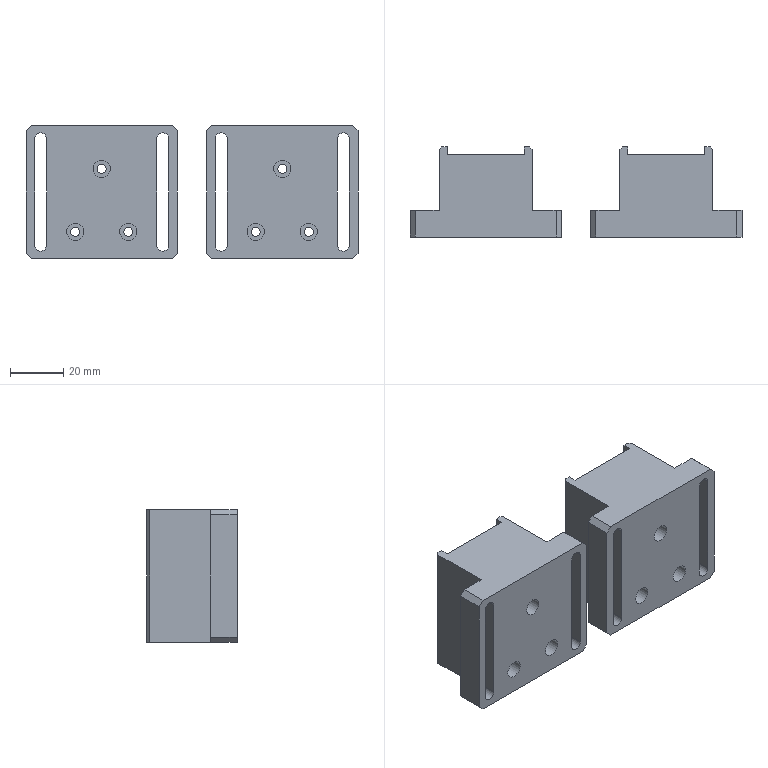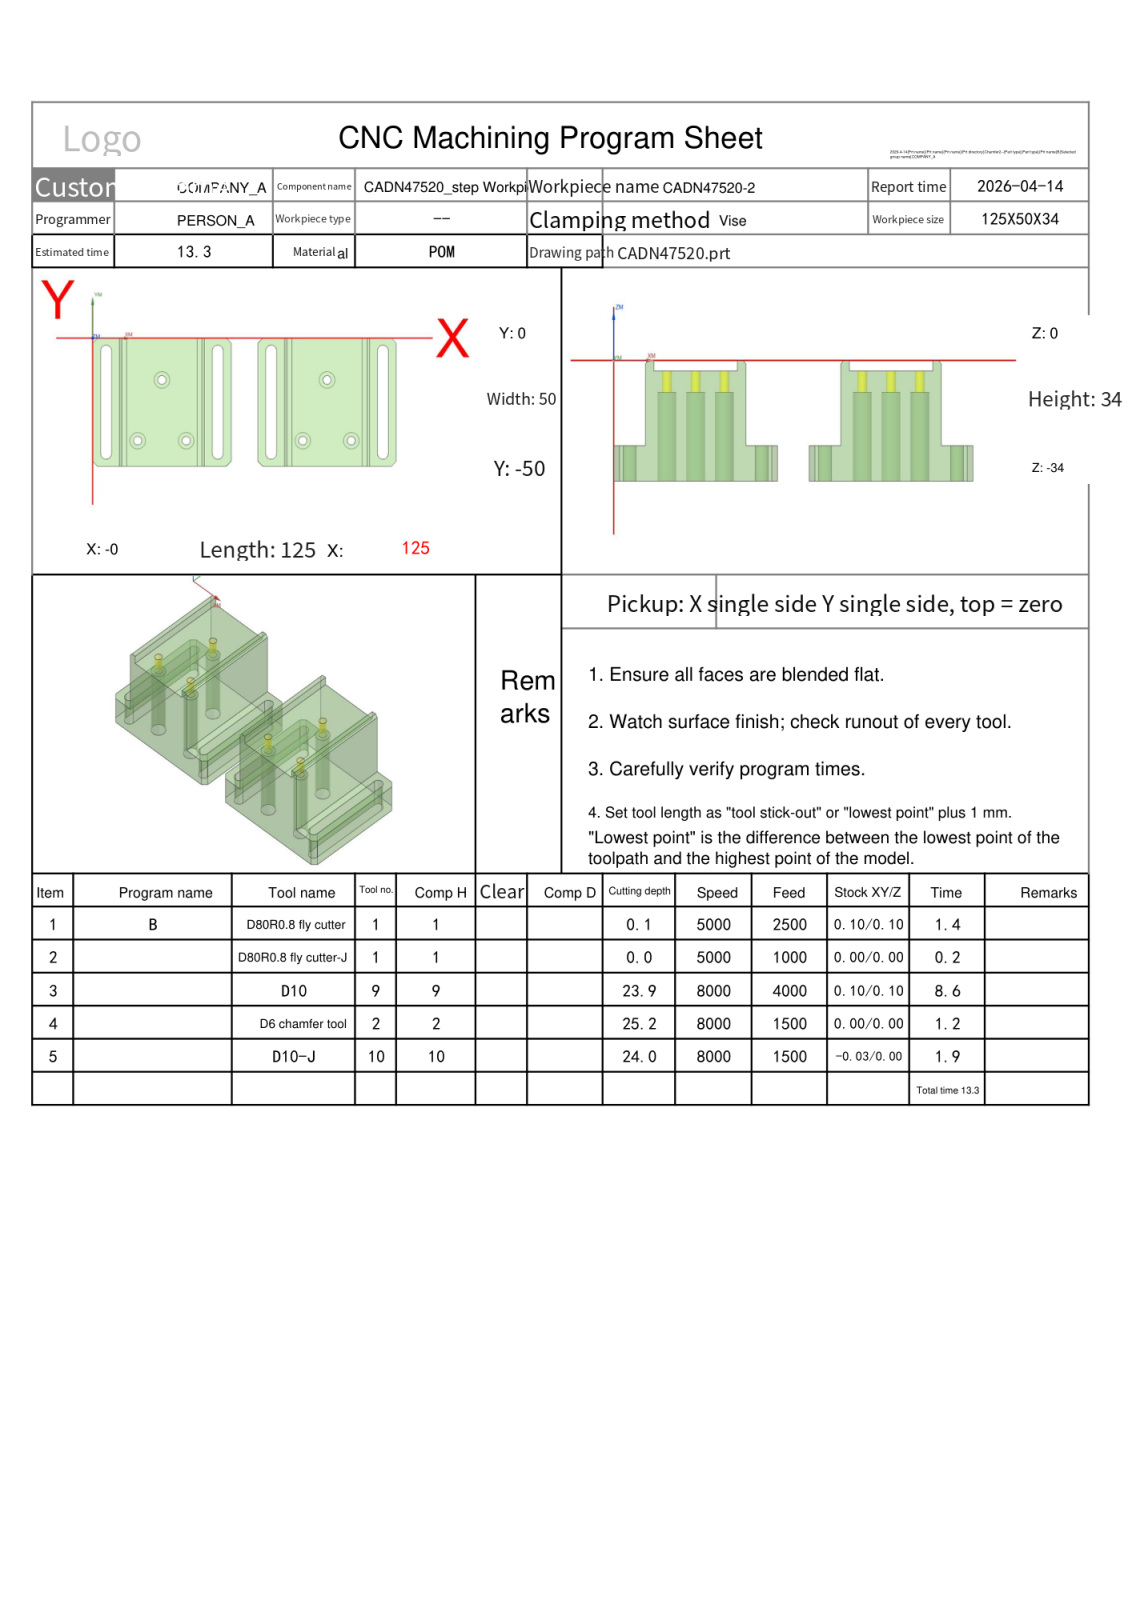NC program | NX | posted by the shop | part box 125 x 34 x 50 mm
Lines 133 to 1886 of 4293:
N3 T09 M06
(D10  D=10. R=0. H=09 ce=0.10 di=0.10)
G00 G90 G54 X28.5 Y-58. M03 S8000
G43 H09 Z15.8
M08
Z.92
G01 Z-.58 F4000.
Y-54.9
X19.1
Y4.9
X37.9
Y-54.9
X31.644
G02 X30.734 Y-54.313 I0.0 J1.
G01 X27.806 Y-47.858
G03 X27.248 Y-47.336 I-.91 J-.414
G02 X26.6 Y-46.402 I.352 J.936
G01 Y-3.598
G02 X27.598 Y-2.6 I1. J-.002
G01 X29.402
G02 X30.4 Y-3.598 I-.002 J-1.
G01 Y-46.402
G02 X29.402 Y-47.4 I-1. J.002
G01 X28.5
X28.
Y-50.4
Y-58.
Z.92
G00 X28.5
Z.34
G01 Z-1.16
Y-54.9
X19.1
Y4.9
X37.9
Y-54.9
X31.644
G02 X30.734 Y-54.313 I0.0 J1.
G01 X27.806 Y-47.858
G03 X27.248 Y-47.336 I-.91 J-.414
G02 X26.6 Y-46.402 I.352 J.936
G01 Y-3.598
G02 X27.598 Y-2.6 I1. J-.002
G01 X29.402
G02 X30.4 Y-3.598 I-.002 J-1.
G01 Y-46.402
G02 X29.402 Y-47.4 I-1. J.002
G01 X28.5
X28.
Y-50.4
Y-58.
Z.34
G00 X28.5
Z-.24
G01 Z-1.74
Y-54.9
X19.1
Y4.9
X37.9
Y-54.9
X31.644
G02 X30.734 Y-54.313 I0.0 J1.
G01 X27.806 Y-47.858
G03 X27.248 Y-47.336 I-.91 J-.414
G02 X26.6 Y-46.402 I.352 J.936
G01 Y-3.598
G02 X27.598 Y-2.6 I1. J-.002
G01 X29.402
G02 X30.4 Y-3.598 I-.002 J-1.
G01 Y-46.402
G02 X29.402 Y-47.4 I-1. J.002
G01 X28.5
X28.
Y-50.4
Y-58.
Z-.24
G00 X28.5
Z-.82
G01 Z-2.32
Y-54.9
X19.1
Y4.9
X37.9
Y-54.9
X31.644
G02 X30.734 Y-54.313 I0.0 J1.
G01 X27.806 Y-47.858
G03 X27.248 Y-47.336 I-.91 J-.414
G02 X26.6 Y-46.402 I.352 J.936
G01 Y-3.598
G02 X27.598 Y-2.6 I1. J-.002
G01 X29.402
G02 X30.4 Y-3.598 I-.002 J-1.
G01 Y-46.402
G02 X29.402 Y-47.4 I-1. J.002
G01 X28.5
X28.
Y-50.4
Y-58.
Z-.82
G00 X28.5
Z-1.4
G01 Z-2.9
Y-54.9
X19.1
Y4.9
X37.9
Y-54.9
X31.644
G02 X30.734 Y-54.313 I0.0 J1.
G01 X27.806 Y-47.858
G03 X27.248 Y-47.336 I-.91 J-.414
G02 X26.6 Y-46.402 I.352 J.936
G01 Y-3.598
G02 X27.598 Y-2.6 I1. J-.002
G01 X29.402
G02 X30.4 Y-3.598 I-.002 J-1.
G01 Y-46.402
G02 X29.402 Y-47.4 I-1. J.002
G01 X28.5
X28.
Y-50.4
Y-58.
Z-1.4
G00 Z3.
X96.5
Z.92
G01 Z-.58
Y-54.9
X87.1
Y4.9
X105.9
Y-54.9
X99.644
G02 X98.734 Y-54.313 I0.0 J1.
G01 X95.806 Y-47.858
G03 X95.248 Y-47.336 I-.91 J-.414
G02 X94.6 Y-46.402 I.352 J.936
G01 Y-3.598
G02 X95.598 Y-2.6 I1. J-.002
G01 X97.402
G02 X98.4 Y-3.598 I-.002 J-1.
G01 Y-46.402
G02 X97.402 Y-47.4 I-1. J.002
G01 X96.5
X96.
Y-50.4
Y-58.
Z.92
G00 X96.5
Z.34
G01 Z-1.16
Y-54.9
X87.1
Y4.9
X105.9
Y-54.9
X99.644
G02 X98.734 Y-54.313 I0.0 J1.
G01 X95.806 Y-47.858
G03 X95.248 Y-47.336 I-.91 J-.414
G02 X94.6 Y-46.402 I.352 J.936
G01 Y-3.598
G02 X95.598 Y-2.6 I1. J-.002
G01 X97.402
G02 X98.4 Y-3.598 I-.002 J-1.
G01 Y-46.402
G02 X97.402 Y-47.4 I-1. J.002
G01 X96.5
X96.
Y-50.4
Y-58.
Z.34
G00 X96.5
Z-.24
G01 Z-1.74
Y-54.9
X87.1
Y4.9
X105.9
Y-54.9
X99.644
G02 X98.734 Y-54.313 I0.0 J1.
G01 X95.806 Y-47.858
G03 X95.248 Y-47.336 I-.91 J-.414
G02 X94.6 Y-46.402 I.352 J.936
G01 Y-3.598
G02 X95.598 Y-2.6 I1. J-.002
G01 X97.402
G02 X98.4 Y-3.598 I-.002 J-1.
G01 Y-46.402
G02 X97.402 Y-47.4 I-1. J.002
G01 X96.5
X96.
Y-50.4
Y-58.
Z-.24
G00 X96.5
Z-.82
G01 Z-2.32
Y-54.9
X87.1
Y4.9
X105.9
Y-54.9
X99.644
G02 X98.734 Y-54.313 I0.0 J1.
G01 X95.806 Y-47.858
G03 X95.248 Y-47.336 I-.91 J-.414
G02 X94.6 Y-46.402 I.352 J.936
G01 Y-3.598
G02 X95.598 Y-2.6 I1. J-.002
G01 X97.402
G02 X98.4 Y-3.598 I-.002 J-1.
G01 Y-46.402
G02 X97.402 Y-47.4 I-1. J.002
G01 X96.5
X96.
Y-50.4
Y-58.
Z-.82
G00 X96.5
Z-1.4
G01 Z-2.9
Y-54.9
X87.1
Y4.9
X105.9
Y-54.9
X99.644
G02 X98.734 Y-54.313 I0.0 J1.
G01 X95.806 Y-47.858
G03 X95.248 Y-47.336 I-.91 J-.414
G02 X94.6 Y-46.402 I.352 J.936
G01 Y-3.598
G02 X95.598 Y-2.6 I1. J-.002
G01 X97.402
G02 X98.4 Y-3.598 I-.002 J-1.
G01 Y-46.402
G02 X97.402 Y-47.4 I-1. J.002
G01 X96.5
X96.
Y-50.4
Y-58.
Z-1.4
G00 Z15.8
G00 G90 X-8. Y-25. M03 S8000
Z15.8
Z.903
G01 Z-.598 F4000.
X-4.9
Y.03
X-.03 Y4.9
X5.9
Y-54.9
X-.03
X-4.9 Y-50.03
Y-27.664
G02 X-4.607 Y-26.957 I1. J0.0
G01 X-.693 Y-23.043
G03 X-.4 Y-22.336 I-.707 J.707
G01 Y-2.205
G02 X.5 Y-1.307 I.9 J-.002
X1.4 Y-2.205 I0.0 J-.9
G01 Y-47.795
G02 X.5 Y-48.693 I-.9 J.002
X-.4 Y-47.795 I0.0 J.9
G01 Y-25.
Y-24.5
X-8.
Z.903
G00 Y-25.
Z.305
G01 Z-1.195
X-4.9
Y.03
X-.03 Y4.9
X5.9
Y-54.9
X-.03
X-4.9 Y-50.03
Y-27.664
G02 X-4.607 Y-26.957 I1. J0.0
G01 X-.693 Y-23.043
G03 X-.4 Y-22.336 I-.707 J.707
G01 Y-2.205
G02 X.5 Y-1.307 I.9 J-.002
X1.4 Y-2.205 I0.0 J-.9
G01 Y-47.795
G02 X.5 Y-48.693 I-.9 J.002
X-.4 Y-47.795 I0.0 J.9
G01 Y-25.
Y-24.5
X-8.
Z.305
G00 Y-25.
Z-.293
G01 Z-1.793
X-4.9
Y.03
X-.03 Y4.9
X5.9
Y-54.9
X-.03
X-4.9 Y-50.03
Y-27.664
G02 X-4.607 Y-26.957 I1. J0.0
G01 X-.693 Y-23.043
G03 X-.4 Y-22.336 I-.707 J.707
G01 Y-2.205
G02 X.5 Y-1.307 I.9 J-.002
X1.4 Y-2.205 I0.0 J-.9
G01 Y-47.795
G02 X.5 Y-48.693 I-.9 J.002
X-.4 Y-47.795 I0.0 J.9
G01 Y-25.
Y-24.5
X-8.
Z-.293
G00 Y-25.
Z-.89
G01 Z-2.39
X-4.9
Y.03
X-.03 Y4.9
X5.9
Y-54.9
X-.03
X-4.9 Y-50.03
Y-27.664
G02 X-4.607 Y-26.957 I1. J0.0
G01 X-.693 Y-23.043
G03 X-.4 Y-22.336 I-.707 J.707
G01 Y-2.205
G02 X.5 Y-1.307 I.9 J-.002
X1.4 Y-2.205 I0.0 J-.9
G01 Y-47.795
G02 X.5 Y-48.693 I-.9 J.002
X-.4 Y-47.795 I0.0 J.9
G01 Y-25.
Y-24.5
X-8.
Z-.89
G00 Y-25.
Z-1.488
G01 Z-2.988
X-4.9
Y.03
X-.03 Y4.9
X5.9
Y-54.9
X-.03
X-4.9 Y-50.03
Y-27.664
G02 X-4.607 Y-26.957 I1. J0.0
G01 X-.693 Y-23.043
G03 X-.4 Y-22.336 I-.707 J.707
G01 Y-2.205
G02 X.5 Y-1.307 I.9 J-.002
X1.4 Y-2.205 I0.0 J-.9
G01 Y-47.795
G02 X.5 Y-48.693 I-.9 J.002
X-.4 Y-47.795 I0.0 J.9
G01 Y-25.
Y-24.5
X-8.
Z-1.488
G00 Y-25.
Z-2.085
G01 Z-3.585
X-4.9
Y.03
X-.03 Y4.9
X5.9
Y-54.9
X-.03
X-4.9 Y-50.03
Y-27.664
G02 X-4.607 Y-26.957 I1. J0.0
G01 X-.693 Y-23.043
G03 X-.4 Y-22.336 I-.707 J.707
G01 Y-2.205
G02 X.5 Y-1.307 I.9 J-.002
X1.4 Y-2.205 I0.0 J-.9
G01 Y-47.795
G02 X.5 Y-48.693 I-.9 J.002
X-.4 Y-47.795 I0.0 J.9
G01 Y-25.
Y-24.5
X-8.
Z-2.085
G00 Y-25.
Z-2.683
G01 Z-4.183
X-4.9
Y.03
X-.03 Y4.9
X5.9
Y-54.9
X-.03
X-4.9 Y-50.03
Y-27.664
G02 X-4.607 Y-26.957 I1. J0.0
G01 X-.693 Y-23.043
G03 X-.4 Y-22.336 I-.707 J.707
G01 Y-2.205
G02 X.5 Y-1.307 I.9 J-.002
X1.4 Y-2.205 I0.0 J-.9
G01 Y-47.795
G02 X.5 Y-48.693 I-.9 J.002
X-.4 Y-47.795 I0.0 J.9
G01 Y-25.
Y-24.5
X-8.
Z-2.683
G00 Y-25.
Z-3.28
G01 Z-4.78
X-4.9
Y.03
X-.03 Y4.9
X5.9
Y-54.9
X-.03
X-4.9 Y-50.03
Y-27.664
G02 X-4.607 Y-26.957 I1. J0.0
G01 X-.693 Y-23.043
G03 X-.4 Y-22.336 I-.707 J.707
G01 Y-2.205
G02 X.5 Y-1.307 I.9 J-.002
X1.4 Y-2.205 I0.0 J-.9
G01 Y-47.795
G02 X.5 Y-48.693 I-.9 J.002
X-.4 Y-47.795 I0.0 J.9
G01 Y-25.
Y-24.5
X-8.
Z-3.28
G00 Y-25.
Z-3.878
G01 Z-5.378
X-4.9
Y.03
X-.03 Y4.9
X5.9
Y-54.9
X-.03
X-4.9 Y-50.03
Y-27.664
G02 X-4.607 Y-26.957 I1. J0.0
G01 X-.693 Y-23.043
G03 X-.4 Y-22.336 I-.707 J.707
G01 Y-2.205
G02 X.5 Y-1.307 I.9 J-.002
X1.4 Y-2.205 I0.0 J-.9
G01 Y-47.795
G02 X.5 Y-48.693 I-.9 J.002
X-.4 Y-47.795 I0.0 J.9
G01 Y-25.
Y-24.5
X-8.
Z-3.878
G00 Y-25.
Z-4.475
G01 Z-5.975
X-4.9
Y.03
X-.03 Y4.9
X5.9
Y-54.9
X-.03
X-4.9 Y-50.03
Y-27.664
G02 X-4.607 Y-26.957 I1. J0.0
G01 X-.693 Y-23.043
G03 X-.4 Y-22.336 I-.707 J.707
G01 Y-2.205
G02 X.5 Y-1.307 I.9 J-.002
X1.4 Y-2.205 I0.0 J-.9
G01 Y-47.795
G02 X.5 Y-48.693 I-.9 J.002
X-.4 Y-47.795 I0.0 J.9
G01 Y-25.
Y-24.5
X-8.
Z-4.475
G00 Y-25.
Z-5.073
G01 Z-6.573
X-4.9
Y.03
X-.03 Y4.9
X5.9
Y-54.9
X-.03
X-4.9 Y-50.03
Y-27.664
G02 X-4.607 Y-26.957 I1. J0.0
G01 X-.693 Y-23.043
G03 X-.4 Y-22.336 I-.707 J.707
G01 Y-2.205
G02 X.5 Y-1.307 I.9 J-.002
X1.4 Y-2.205 I0.0 J-.9
G01 Y-47.795
G02 X.5 Y-48.693 I-.9 J.002
X-.4 Y-47.795 I0.0 J.9
G01 Y-25.
Y-24.5
X-8.
Z-5.073
G00 Y-25.
Z-5.67
G01 Z-7.17
X-4.9
Y.03
X-.03 Y4.9
X5.9
Y-54.9
X-.03
X-4.9 Y-50.03
Y-27.664
G02 X-4.607 Y-26.957 I1. J0.0
G01 X-.693 Y-23.043
G03 X-.4 Y-22.336 I-.707 J.707
G01 Y-2.205
G02 X.5 Y-1.307 I.9 J-.002
X1.4 Y-2.205 I0.0 J-.9
G01 Y-47.795
G02 X.5 Y-48.693 I-.9 J.002
X-.4 Y-47.795 I0.0 J.9
G01 Y-25.
Y-24.5
X-8.
Z-5.67
G00 Y-25.
Z-6.268
G01 Z-7.768
X-4.9
Y.03
X-.03 Y4.9
X5.9
Y-54.9
X-.03
X-4.9 Y-50.03
Y-27.664
G02 X-4.607 Y-26.957 I1. J0.0
G01 X-.693 Y-23.043
G03 X-.4 Y-22.336 I-.707 J.707
G01 Y-2.205
G02 X.5 Y-1.307 I.9 J-.002
X1.4 Y-2.205 I0.0 J-.9
G01 Y-47.795
G02 X.5 Y-48.693 I-.9 J.002
X-.4 Y-47.795 I0.0 J.9
G01 Y-25.
Y-24.5
X-8.
Z-6.268
G00 Y-25.
Z-6.865
G01 Z-8.365
X-4.9
Y.03
X-.03 Y4.9
X5.9
Y-54.9
X-.03
X-4.9 Y-50.03
Y-27.664
G02 X-4.607 Y-26.957 I1. J0.0
G01 X-.693 Y-23.043
G03 X-.4 Y-22.336 I-.707 J.707
G01 Y-2.205
G02 X.5 Y-1.307 I.9 J-.002
X1.4 Y-2.205 I0.0 J-.9
G01 Y-47.795
G02 X.5 Y-48.693 I-.9 J.002
X-.4 Y-47.795 I0.0 J.9
G01 Y-25.
Y-24.5
X-8.
Z-6.865
G00 Y-25.
Z-7.463
G01 Z-8.963
X-4.9
Y.03
X-.03 Y4.9
X5.9
Y-54.9
X-.03
X-4.9 Y-50.03
Y-27.664
G02 X-4.607 Y-26.957 I1. J0.0
G01 X-.693 Y-23.043
G03 X-.4 Y-22.336 I-.707 J.707
G01 Y-2.205
G02 X.5 Y-1.307 I.9 J-.002
X1.4 Y-2.205 I0.0 J-.9
G01 Y-47.795
G02 X.5 Y-48.693 I-.9 J.002
X-.4 Y-47.795 I0.0 J.9
G01 Y-25.
Y-24.5
X-8.
Z-7.463
G00 Y-25.
Z-8.06
G01 Z-9.56
X-4.9
Y.03
X-.03 Y4.9
X5.9
Y-54.9
X-.03
X-4.9 Y-50.03
Y-27.664
G02 X-4.607 Y-26.957 I1. J0.0
G01 X-.693 Y-23.043
G03 X-.4 Y-22.336 I-.707 J.707
G01 Y-2.205
G02 X.5 Y-1.307 I.9 J-.002
X1.4 Y-2.205 I0.0 J-.9
G01 Y-47.795
G02 X.5 Y-48.693 I-.9 J.002
X-.4 Y-47.795 I0.0 J.9
G01 Y-25.
Y-24.5
X-8.
Z-8.06
G00 Y-25.
Z-8.658
G01 Z-10.158
X-4.9
Y.03
X-.03 Y4.9
X5.9
Y-54.9
X-.03
X-4.9 Y-50.03
Y-27.664
G02 X-4.607 Y-26.957 I1. J0.0
G01 X-.693 Y-23.043
G03 X-.4 Y-22.336 I-.707 J.707
G01 Y-2.205
G02 X.5 Y-1.307 I.9 J-.002
X1.4 Y-2.205 I0.0 J-.9
G01 Y-47.795
G02 X.5 Y-48.693 I-.9 J.002
X-.4 Y-47.795 I0.0 J.9
G01 Y-25.
Y-24.5
X-8.
Z-8.658
G00 Y-25.
Z-9.255
G01 Z-10.755
X-4.9
Y.03
X-.03 Y4.9
X5.9
Y-54.9
X-.03
X-4.9 Y-50.03
Y-27.664
G02 X-4.607 Y-26.957 I1. J0.0
G01 X-.693 Y-23.043
G03 X-.4 Y-22.336 I-.707 J.707
G01 Y-2.205
G02 X.5 Y-1.307 I.9 J-.002
X1.4 Y-2.205 I0.0 J-.9
G01 Y-47.795
G02 X.5 Y-48.693 I-.9 J.002
X-.4 Y-47.795 I0.0 J.9
G01 Y-25.
Y-24.5
X-8.
Z-9.255
G00 Y-25.
Z-9.853
G01 Z-11.353
X-4.9
Y.03
X-.03 Y4.9
X5.9
Y-54.9
X-.03
X-4.9 Y-50.03
Y-27.664
G02 X-4.607 Y-26.957 I1. J0.0
G01 X-.693 Y-23.043
G03 X-.4 Y-22.336 I-.707 J.707
G01 Y-2.205
G02 X.5 Y-1.307 I.9 J-.002
X1.4 Y-2.205 I0.0 J-.9
G01 Y-47.795
G02 X.5 Y-48.693 I-.9 J.002
X-.4 Y-47.795 I0.0 J.9
G01 Y-25.
Y-24.5
X-8.
Z-9.853
G00 Y-25.
Z-10.45
G01 Z-11.95
X-4.9
Y.03
X-.03 Y4.9
X5.9
Y-54.9
X-.03
X-4.9 Y-50.03
Y-27.664
G02 X-4.607 Y-26.957 I1. J0.0
G01 X-.693 Y-23.043
G03 X-.4 Y-22.336 I-.707 J.707
G01 Y-2.205
G02 X.5 Y-1.307 I.9 J-.002
X1.4 Y-2.205 I0.0 J-.9
G01 Y-47.795
G02 X.5 Y-48.693 I-.9 J.002
X-.4 Y-47.795 I0.0 J.9
G01 Y-25.
Y-24.5
X-8.
Z-10.45
G00 Y-25.
Z-11.048
G01 Z-12.548
X-4.9
Y.03
X-.03 Y4.9
X5.9
Y-54.9
X-.03
X-4.9 Y-50.03
Y-27.664
G02 X-4.607 Y-26.957 I1. J0.0
G01 X-.693 Y-23.043
G03 X-.4 Y-22.336 I-.707 J.707
G01 Y-2.205
G02 X.5 Y-1.307 I.9 J-.002
X1.4 Y-2.205 I0.0 J-.9
G01 Y-47.795
G02 X.5 Y-48.693 I-.9 J.002
X-.4 Y-47.795 I0.0 J.9
G01 Y-25.
Y-24.5
X-8.
Z-11.048
G00 Y-25.
Z-11.645
G01 Z-13.145
X-4.9
Y.03
X-.03 Y4.9
X5.9
Y-54.9
X-.03
X-4.9 Y-50.03
Y-27.664
G02 X-4.607 Y-26.957 I1. J0.0
G01 X-.693 Y-23.043
G03 X-.4 Y-22.336 I-.707 J.707
G01 Y-2.205
G02 X.5 Y-1.307 I.9 J-.002
X1.4 Y-2.205 I0.0 J-.9
G01 Y-47.795
G02 X.5 Y-48.693 I-.9 J.002
X-.4 Y-47.795 I0.0 J.9
G01 Y-25.
Y-24.5
X-8.
Z-11.645
G00 Y-25.
Z-12.243
G01 Z-13.743
X-4.9
Y.03
X-.03 Y4.9
X5.9
Y-54.9
X-.03
X-4.9 Y-50.03
Y-27.664
G02 X-4.607 Y-26.957 I1. J0.0
G01 X-.693 Y-23.043
G03 X-.4 Y-22.336 I-.707 J.707
G01 Y-2.205
G02 X.5 Y-1.307 I.9 J-.002
X1.4 Y-2.205 I0.0 J-.9
G01 Y-47.795
G02 X.5 Y-48.693 I-.9 J.002
X-.4 Y-47.795 I0.0 J.9
G01 Y-25.
Y-24.5
X-8.
Z-12.243
G00 Y-25.
Z-12.84
G01 Z-14.34
X-4.9
Y.03
X-.03 Y4.9
X5.9
Y-54.9
X-.03
X-4.9 Y-50.03
Y-27.664
G02 X-4.607 Y-26.957 I1. J0.0
G01 X-.693 Y-23.043
G03 X-.4 Y-22.336 I-.707 J.707
G01 Y-2.205
G02 X.5 Y-1.307 I.9 J-.002
X1.4 Y-2.205 I0.0 J-.9
G01 Y-47.795
G02 X.5 Y-48.693 I-.9 J.002
X-.4 Y-47.795 I0.0 J.9
G01 Y-25.
Y-24.5
X-8.
Z-12.84
G00 Y-25.
Z-13.438
G01 Z-14.938
X-4.9
Y.03
X-.03 Y4.9
X5.9
Y-54.9
X-.03
X-4.9 Y-50.03
Y-27.664
G02 X-4.607 Y-26.957 I1. J0.0
G01 X-.693 Y-23.043
G03 X-.4 Y-22.336 I-.707 J.707
G01 Y-2.205
G02 X.5 Y-1.307 I.9 J-.002
X1.4 Y-2.205 I0.0 J-.9
G01 Y-47.795
G02 X.5 Y-48.693 I-.9 J.002
X-.4 Y-47.795 I0.0 J.9
G01 Y-25.
Y-24.5
X-8.
Z-13.438
G00 Y-25.
Z-14.035
G01 Z-15.535
X-4.9
Y.03
X-.03 Y4.9
X5.9
Y-54.9
X-.03
X-4.9 Y-50.03
Y-27.664
G02 X-4.607 Y-26.957 I1. J0.0
G01 X-.693 Y-23.043
G03 X-.4 Y-22.336 I-.707 J.707
G01 Y-2.205
G02 X.5 Y-1.307 I.9 J-.002
X1.4 Y-2.205 I0.0 J-.9
G01 Y-47.795
G02 X.5 Y-48.693 I-.9 J.002
X-.4 Y-47.795 I0.0 J.9
G01 Y-25.
Y-24.5
X-8.
Z-14.035
G00 Y-25.
Z-14.633
G01 Z-16.133
X-4.9
Y.03
X-.03 Y4.9
X5.9
Y-54.9
X-.03
X-4.9 Y-50.03
Y-27.664
G02 X-4.607 Y-26.957 I1. J0.0
G01 X-.693 Y-23.043
G03 X-.4 Y-22.336 I-.707 J.707
G01 Y-2.205
G02 X.5 Y-1.307 I.9 J-.002
X1.4 Y-2.205 I0.0 J-.9
G01 Y-47.795
G02 X.5 Y-48.693 I-.9 J.002
X-.4 Y-47.795 I0.0 J.9
G01 Y-25.
Y-24.5
X-8.
Z-14.633
G00 Y-25.
Z-15.23
G01 Z-16.73
X-4.9
Y.03
X-.03 Y4.9
X5.9
Y-54.9
X-.03
X-4.9 Y-50.03
Y-27.664
G02 X-4.607 Y-26.957 I1. J0.0
G01 X-.693 Y-23.043
G03 X-.4 Y-22.336 I-.707 J.707
G01 Y-2.205
G02 X.5 Y-1.307 I.9 J-.002
X1.4 Y-2.205 I0.0 J-.9
G01 Y-47.795
G02 X.5 Y-48.693 I-.9 J.002
X-.4 Y-47.795 I0.0 J.9
G01 Y-25.
Y-24.5
X-8.
Z-15.23
G00 Y-25.
Z-15.828
G01 Z-17.328
X-4.9
Y.03
X-.03 Y4.9
X5.9
Y-54.9
X-.03
X-4.9 Y-50.03
Y-27.664
G02 X-4.607 Y-26.957 I1. J0.0
G01 X-.693 Y-23.043
G03 X-.4 Y-22.336 I-.707 J.707
G01 Y-2.205
G02 X.5 Y-1.307 I.9 J-.002
X1.4 Y-2.205 I0.0 J-.9
G01 Y-47.795
G02 X.5 Y-48.693 I-.9 J.002
X-.4 Y-47.795 I0.0 J.9
G01 Y-25.
Y-24.5
X-8.
Z-15.828
G00 Y-25.
Z-16.425
G01 Z-17.925
X-4.9
Y.03
X-.03 Y4.9
X5.9
Y-54.9
X-.03
X-4.9 Y-50.03
Y-27.664
G02 X-4.607 Y-26.957 I1. J0.0
G01 X-.693 Y-23.043
G03 X-.4 Y-22.336 I-.707 J.707
G01 Y-2.205
G02 X.5 Y-1.307 I.9 J-.002
X1.4 Y-2.205 I0.0 J-.9
G01 Y-47.795
G02 X.5 Y-48.693 I-.9 J.002
X-.4 Y-47.795 I0.0 J.9
G01 Y-25.
Y-24.5
X-8.
Z-16.425
G00 Y-25.
Z-17.023
G01 Z-18.523
X-4.9
Y.03
X-.03 Y4.9
X5.9
Y-54.9
X-.03
X-4.9 Y-50.03
Y-27.664
G02 X-4.607 Y-26.957 I1. J0.0
G01 X-.693 Y-23.043
G03 X-.4 Y-22.336 I-.707 J.707
G01 Y-2.205
G02 X.5 Y-1.307 I.9 J-.002
X1.4 Y-2.205 I0.0 J-.9
G01 Y-47.795
G02 X.5 Y-48.693 I-.9 J.002
X-.4 Y-47.795 I0.0 J.9
G01 Y-25.
Y-24.5
X-8.
Z-17.023
G00 Y-25.
Z-17.62
G01 Z-19.12
X-4.9
Y.03
X-.03 Y4.9
X5.9
Y-54.9
X-.03
X-4.9 Y-50.03
Y-27.664
G02 X-4.607 Y-26.957 I1. J0.0
G01 X-.693 Y-23.043
G03 X-.4 Y-22.336 I-.707 J.707
G01 Y-2.205
G02 X.5 Y-1.307 I.9 J-.002
X1.4 Y-2.205 I0.0 J-.9
G01 Y-47.795
G02 X.5 Y-48.693 I-.9 J.002
X-.4 Y-47.795 I0.0 J.9
G01 Y-25.
Y-24.5
X-8.
Z-17.62
G00 Y-25.
Z-18.218
G01 Z-19.718
X-4.9
Y.03
X-.03 Y4.9
X5.9
Y-54.9
X-.03
X-4.9 Y-50.03
Y-27.664
G02 X-4.607 Y-26.957 I1. J0.0
G01 X-.693 Y-23.043
G03 X-.4 Y-22.336 I-.707 J.707
G01 Y-2.205
G02 X.5 Y-1.307 I.9 J-.002
X1.4 Y-2.205 I0.0 J-.9
G01 Y-47.795
G02 X.5 Y-48.693 I-.9 J.002
X-.4 Y-47.795 I0.0 J.9
G01 Y-25.
Y-24.5
X-8.
Z-18.218
G00 Y-25.
Z-18.815
G01 Z-20.315
X-4.9
Y.03
X-.03 Y4.9
X5.9
Y-54.9
X-.03
X-4.9 Y-50.03
Y-27.664
G02 X-4.607 Y-26.957 I1. J0.0
G01 X-.693 Y-23.043
G03 X-.4 Y-22.336 I-.707 J.707
G01 Y-2.205
G02 X.5 Y-1.307 I.9 J-.002
X1.4 Y-2.205 I0.0 J-.9
G01 Y-47.795
G02 X.5 Y-48.693 I-.9 J.002
X-.4 Y-47.795 I0.0 J.9
G01 Y-25.
Y-24.5
X-8.
Z-18.815
G00 Y-25.
Z-19.413
G01 Z-20.913
X-4.9
Y.03
X-.03 Y4.9
X5.9
Y-54.9
X-.03
X-4.9 Y-50.03
Y-27.664
G02 X-4.607 Y-26.957 I1. J0.0
G01 X-.693 Y-23.043
G03 X-.4 Y-22.336 I-.707 J.707
G01 Y-2.205
G02 X.5 Y-1.307 I.9 J-.002
X1.4 Y-2.205 I0.0 J-.9
G01 Y-47.795
G02 X.5 Y-48.693 I-.9 J.002
X-.4 Y-47.795 I0.0 J.9
G01 Y-25.
Y-24.5
X-8.
Z-19.413
G00 Y-25.
Z-20.01
G01 Z-21.51
X-4.9
Y.03
X-.03 Y4.9
X5.9
Y-54.9
X-.03
X-4.9 Y-50.03
Y-27.664
G02 X-4.607 Y-26.957 I1. J0.0
G01 X-.693 Y-23.043
G03 X-.4 Y-22.336 I-.707 J.707
G01 Y-2.205
G02 X.5 Y-1.307 I.9 J-.002
X1.4 Y-2.205 I0.0 J-.9
G01 Y-47.795
G02 X.5 Y-48.693 I-.9 J.002
X-.4 Y-47.795 I0.0 J.9
G01 Y-25.
Y-24.5
X-8.
Z-20.01
G00 Y-25.
Z-20.608
G01 Z-22.108
X-4.9
Y.03
X-.03 Y4.9
X5.9
Y-54.9
X-.03
X-4.9 Y-50.03
Y-27.664
G02 X-4.607 Y-26.957 I1. J0.0
G01 X-.693 Y-23.043
G03 X-.4 Y-22.336 I-.707 J.707
G01 Y-2.205
G02 X.5 Y-1.307 I.9 J-.002
X1.4 Y-2.205 I0.0 J-.9
G01 Y-47.795
G02 X.5 Y-48.693 I-.9 J.002
X-.4 Y-47.795 I0.0 J.9
G01 Y-25.
Y-24.5
X-8.
Z-20.608
G00 Y-25.
Z-21.205
G01 Z-22.705
X-4.9
Y.03
X-.03 Y4.9
X5.9
Y-54.9
X-.03
X-4.9 Y-50.03
Y-27.664
G02 X-4.607 Y-26.957 I1. J0.0
G01 X-.693 Y-23.043
G03 X-.4 Y-22.336 I-.707 J.707
G01 Y-2.205
G02 X.5 Y-1.307 I.9 J-.002
X1.4 Y-2.205 I0.0 J-.9
G01 Y-47.795
G02 X.5 Y-48.693 I-.9 J.002
X-.4 Y-47.795 I0.0 J.9
G01 Y-25.
Y-24.5
X-8.
Z-21.205
G00 Y-25.
Z-21.803
G01 Z-23.303
X-4.9
Y.03
X-.03 Y4.9
X5.9
Y-54.9
X-.03
X-4.9 Y-50.03
Y-27.664
G02 X-4.607 Y-26.957 I1. J0.0
G01 X-.693 Y-23.043
G03 X-.4 Y-22.336 I-.707 J.707
G01 Y-2.205
G02 X.5 Y-1.307 I.9 J-.002
X1.4 Y-2.205 I0.0 J-.9
G01 Y-47.795
G02 X.5 Y-48.693 I-.9 J.002
X-.4 Y-47.795 I0.0 J.9
G01 Y-25.
Y-24.5
X-8.
Z-21.803
G00 Y-25.
Z-22.4
G01 Z-23.9
X-4.9
Y.03
X-.03 Y4.9
X5.9
Y-54.9
X-.03
X-4.9 Y-50.03
Y-27.664
G02 X-4.607 Y-26.957 I1. J0.0
G01 X-.693 Y-23.043
G03 X-.4 Y-22.336 I-.707 J.707
G01 Y-2.205
G02 X.5 Y-1.307 I.9 J-.002
X1.4 Y-2.205 I0.0 J-.9
G01 Y-47.795
G02 X.5 Y-48.693 I-.9 J.002
X-.4 Y-47.795 I0.0 J.9
G01 Y-25.
Y-24.5
X-8.
Z-22.4
G00 Z15.8
X62.5 Y7.57
Z.903
G01 Z-.598
Y4.47
X67.54
X67.97 Y4.9
X73.9
Y-54.9
X67.97
X67.54 Y-54.47
X57.46
X57.03 Y-54.9
X51.1
Y4.9
X57.03
X57.46 Y4.47
X59.465
G02 X60.297 Y4.025 I0.0 J-1.
G01 X64.707 Y-2.59
G03 X65.469 Y-3.033 I.832 J.555
G02 X66.4 Y-4.028 I-.069 J-.998
G01 Y-45.972
G02 X65.402 Y-46.97 I-1. J.002
G01 X59.598
G02 X58.6 Y-45.972 I.002 J1.
G01 Y-4.028
G02 X59.598 Y-3.03 I1. J-.002
G01 X62.5
X63.
Y-.03
Y7.57
Z.903
G00 X62.5
Z.305
G01 Z-1.195
Y4.47
X67.54
X67.97 Y4.9
X73.9
Y-54.9
X67.97
X67.54 Y-54.47
X57.46
X57.03 Y-54.9
X51.1
Y4.9
X57.03
X57.46 Y4.47
X59.465
G02 X60.297 Y4.025 I0.0 J-1.
G01 X64.707 Y-2.59
G03 X65.469 Y-3.033 I.832 J.555
G02 X66.4 Y-4.028 I-.069 J-.998
G01 Y-45.972
G02 X65.402 Y-46.97 I-1. J.002
G01 X59.598
G02 X58.6 Y-45.972 I.002 J1.
G01 Y-4.028
G02 X59.598 Y-3.03 I1. J-.002
G01 X62.5
X63.
Y-.03
Y7.57
Z.305
G00 X62.5
Z-.293
G01 Z-1.793
Y4.47
X67.54
X67.97 Y4.9
X73.9
Y-54.9
X67.97
X67.54 Y-54.47
X57.46
X57.03 Y-54.9
X51.1
Y4.9
X57.03
X57.46 Y4.47
X59.465
G02 X60.297 Y4.025 I0.0 J-1.
G01 X64.707 Y-2.59
G03 X65.469 Y-3.033 I.832 J.555
G02 X66.4 Y-4.028 I-.069 J-.998
G01 Y-45.972
G02 X65.402 Y-46.97 I-1. J.002
G01 X59.598
G02 X58.6 Y-45.972 I.002 J1.
G01 Y-4.028
G02 X59.598 Y-3.03 I1. J-.002
G01 X62.5
X63.
Y-.03
Y7.57
Z-.293
G00 X62.5
Z-.89
G01 Z-2.39
Y4.47
X67.54
X67.97 Y4.9
X73.9
Y-54.9
X67.97
X67.54 Y-54.47
X57.46
X57.03 Y-54.9
X51.1
Y4.9
X57.03
X57.46 Y4.47
X59.465
G02 X60.297 Y4.025 I0.0 J-1.
G01 X64.707 Y-2.59
G03 X65.469 Y-3.033 I.832 J.555
G02 X66.4 Y-4.028 I-.069 J-.998
G01 Y-45.972
G02 X65.402 Y-46.97 I-1. J.002
G01 X59.598
G02 X58.6 Y-45.972 I.002 J1.
G01 Y-4.028
G02 X59.598 Y-3.03 I1. J-.002
G01 X62.5
X63.
Y-.03
Y7.57
Z-.89
G00 X62.5
Z-1.488
G01 Z-2.988
Y4.47
X67.54
X67.97 Y4.9
X73.9
Y-54.9
X67.97
X67.54 Y-54.47
X57.46
X57.03 Y-54.9
X51.1
Y4.9
X57.03
X57.46 Y4.47
X59.465
G02 X60.297 Y4.025 I0.0 J-1.
G01 X64.707 Y-2.59
G03 X65.469 Y-3.033 I.832 J.555
G02 X66.4 Y-4.028 I-.069 J-.998
G01 Y-45.972
G02 X65.402 Y-46.97 I-1. J.002
G01 X59.598
G02 X58.6 Y-45.972 I.002 J1.
G01 Y-4.028
G02 X59.598 Y-3.03 I1. J-.002
G01 X62.5
X63.
Y-.03
Y7.57
Z-1.488
G00 X62.5
Z-2.085
G01 Z-3.585
Y4.47
X67.54
X67.97 Y4.9
X73.9
Y-54.9
X67.97
X67.54 Y-54.47
X57.46
X57.03 Y-54.9
X51.1
Y4.9
X57.03
X57.46 Y4.47
X59.465
G02 X60.297 Y4.025 I0.0 J-1.
G01 X64.707 Y-2.59
G03 X65.469 Y-3.033 I.832 J.555
G02 X66.4 Y-4.028 I-.069 J-.998
G01 Y-45.972
G02 X65.402 Y-46.97 I-1. J.002
G01 X59.598
G02 X58.6 Y-45.972 I.002 J1.
G01 Y-4.028
G02 X59.598 Y-3.03 I1. J-.002
G01 X62.5
X63.
Y-.03
Y7.57
Z-2.085
G00 X62.5
Z-2.683
G01 Z-4.183
Y4.47
X67.54
X67.97 Y4.9
X73.9
Y-54.9
X67.97
X67.54 Y-54.47
X57.46
X57.03 Y-54.9
X51.1
Y4.9
X57.03
X57.46 Y4.47
X59.465
G02 X60.297 Y4.025 I0.0 J-1.
G01 X64.707 Y-2.59
G03 X65.469 Y-3.033 I.832 J.555
G02 X66.4 Y-4.028 I-.069 J-.998
G01 Y-45.972
G02 X65.402 Y-46.97 I-1. J.002
G01 X59.598
G02 X58.6 Y-45.972 I.002 J1.
G01 Y-4.028
G02 X59.598 Y-3.03 I1. J-.002
G01 X62.5
X63.
Y-.03
Y7.57
Z-2.683
G00 X62.5
Z-3.28
G01 Z-4.78
Y4.47
X67.54
X67.97 Y4.9
X73.9
Y-54.9
X67.97
X67.54 Y-54.47
X57.46
X57.03 Y-54.9
X51.1
Y4.9
X57.03
X57.46 Y4.47
X59.465
G02 X60.297 Y4.025 I0.0 J-1.
G01 X64.707 Y-2.59
G03 X65.469 Y-3.033 I.832 J.555
G02 X66.4 Y-4.028 I-.069 J-.998
G01 Y-45.972
G02 X65.402 Y-46.97 I-1. J.002
G01 X59.598
G02 X58.6 Y-45.972 I.002 J1.
G01 Y-4.028
G02 X59.598 Y-3.03 I1. J-.002
G01 X62.5
X63.
Y-.03
Y7.57
Z-3.28
G00 X62.5
Z-3.878
G01 Z-5.378
Y4.47
X67.54
X67.97 Y4.9
X73.9
Y-54.9
X67.97
X67.54 Y-54.47
X57.46
X57.03 Y-54.9
X51.1
Y4.9
X57.03
X57.46 Y4.47
X59.465
G02 X60.297 Y4.025 I0.0 J-1.
G01 X64.707 Y-2.59
G03 X65.469 Y-3.033 I.832 J.555
G02 X66.4 Y-4.028 I-.069 J-.998
G01 Y-45.972
G02 X65.402 Y-46.97 I-1. J.002
G01 X59.598
G02 X58.6 Y-45.972 I.002 J1.
G01 Y-4.028
G02 X59.598 Y-3.03 I1. J-.002
G01 X62.5
X63.
Y-.03
Y7.57
Z-3.878
G00 X62.5
Z-4.475
G01 Z-5.975
Y4.47
X67.54
X67.97 Y4.9
X73.9
Y-54.9
X67.97
X67.54 Y-54.47
X57.46
X57.03 Y-54.9
X51.1
Y4.9
X57.03
X57.46 Y4.47
X59.465
G02 X60.297 Y4.025 I0.0 J-1.
G01 X64.707 Y-2.59
G03 X65.469 Y-3.033 I.832 J.555
G02 X66.4 Y-4.028 I-.069 J-.998
G01 Y-45.972
G02 X65.402 Y-46.97 I-1. J.002
G01 X59.598
G02 X58.6 Y-45.972 I.002 J1.
G01 Y-4.028
G02 X59.598 Y-3.03 I1. J-.002
G01 X62.5
X63.
Y-.03
Y7.57
Z-4.475
G00 X62.5
Z-5.073
G01 Z-6.573
Y4.47
X67.54
X67.97 Y4.9
X73.9
Y-54.9
X67.97
X67.54 Y-54.47
X57.46
X57.03 Y-54.9
X51.1
Y4.9
X57.03
X57.46 Y4.47
X59.465
G02 X60.297 Y4.025 I0.0 J-1.
G01 X64.707 Y-2.59
G03 X65.469 Y-3.033 I.832 J.555
G02 X66.4 Y-4.028 I-.069 J-.998
G01 Y-45.972
G02 X65.402 Y-46.97 I-1. J.002
G01 X59.598
G02 X58.6 Y-45.972 I.002 J1.
G01 Y-4.028
G02 X59.598 Y-3.03 I1. J-.002
G01 X62.5
X63.
Y-.03
Y7.57
Z-5.073
G00 X62.5
Z-5.67
G01 Z-7.17
Y4.47
X67.54
X67.97 Y4.9
X73.9
Y-54.9
X67.97
X67.54 Y-54.47
X57.46
X57.03 Y-54.9
X51.1
Y4.9
X57.03
X57.46 Y4.47
X59.465
G02 X60.297 Y4.025 I0.0 J-1.
G01 X64.707 Y-2.59
G03 X65.469 Y-3.033 I.832 J.555
G02 X66.4 Y-4.028 I-.069 J-.998
G01 Y-45.972
G02 X65.402 Y-46.97 I-1. J.002
G01 X59.598
G02 X58.6 Y-45.972 I.002 J1.
G01 Y-4.028
G02 X59.598 Y-3.03 I1. J-.002
G01 X62.5
X63.
Y-.03
Y7.57
Z-5.67
G00 X62.5
Z-6.268
G01 Z-7.768
Y4.47
X67.54
X67.97 Y4.9
X73.9
Y-54.9
X67.97
X67.54 Y-54.47
X57.46
X57.03 Y-54.9
X51.1
Y4.9
X57.03
X57.46 Y4.47
X59.465
G02 X60.297 Y4.025 I0.0 J-1.
G01 X64.707 Y-2.59
G03 X65.469 Y-3.033 I.832 J.555
G02 X66.4 Y-4.028 I-.069 J-.998
G01 Y-45.972
G02 X65.402 Y-46.97 I-1. J.002
G01 X59.598
G02 X58.6 Y-45.972 I.002 J1.
G01 Y-4.028
G02 X59.598 Y-3.03 I1. J-.002
G01 X62.5
X63.
Y-.03
Y7.57
Z-6.268
G00 X62.5
Z-6.865
G01 Z-8.365
Y4.47
X67.54
X67.97 Y4.9
X73.9
Y-54.9
X67.97
X67.54 Y-54.47
X57.46
X57.03 Y-54.9
X51.1
Y4.9
X57.03
X57.46 Y4.47
X59.465
G02 X60.297 Y4.025 I0.0 J-1.
G01 X64.707 Y-2.59
G03 X65.469 Y-3.033 I.832 J.555
G02 X66.4 Y-4.028 I-.069 J-.998
G01 Y-45.972
G02 X65.402 Y-46.97 I-1. J.002
G01 X59.598
G02 X58.6 Y-45.972 I.002 J1.
G01 Y-4.028
G02 X59.598 Y-3.03 I1. J-.002
G01 X62.5
X63.
Y-.03
Y7.57
Z-6.865
G00 X62.5
Z-7.463
G01 Z-8.963
Y4.47
X67.54
X67.97 Y4.9
X73.9
Y-54.9
X67.97
X67.54 Y-54.47
X57.46
X57.03 Y-54.9
X51.1
Y4.9
X57.03
X57.46 Y4.47
X59.465
G02 X60.297 Y4.025 I0.0 J-1.
G01 X64.707 Y-2.59
G03 X65.469 Y-3.033 I.832 J.555
G02 X66.4 Y-4.028 I-.069 J-.998
G01 Y-45.972
G02 X65.402 Y-46.97 I-1. J.002
G01 X59.598
G02 X58.6 Y-45.972 I.002 J1.
G01 Y-4.028
G02 X59.598 Y-3.03 I1. J-.002
G01 X62.5
X63.
Y-.03
Y7.57
Z-7.463
G00 X62.5
Z-8.06
G01 Z-9.56
Y4.47
X67.54
X67.97 Y4.9
X73.9
Y-54.9
X67.97
X67.54 Y-54.47
X57.46
X57.03 Y-54.9
X51.1
Y4.9
X57.03
X57.46 Y4.47
X59.465
G02 X60.297 Y4.025 I0.0 J-1.
G01 X64.707 Y-2.59
G03 X65.469 Y-3.033 I.832 J.555
G02 X66.4 Y-4.028 I-.069 J-.998
G01 Y-45.972
G02 X65.402 Y-46.97 I-1. J.002
G01 X59.598
G02 X58.6 Y-45.972 I.002 J1.
G01 Y-4.028
G02 X59.598 Y-3.03 I1. J-.002
G01 X62.5
X63.
Y-.03
Y7.57
Z-8.06
G00 X62.5
Z-8.658
G01 Z-10.158
Y4.47
X67.54
X67.97 Y4.9
X73.9
Y-54.9
X67.97
X67.54 Y-54.47
X57.46
X57.03 Y-54.9
X51.1
Y4.9
X57.03
X57.46 Y4.47
X59.465
G02 X60.297 Y4.025 I0.0 J-1.
G01 X64.707 Y-2.59
G03 X65.469 Y-3.033 I.832 J.555
G02 X66.4 Y-4.028 I-.069 J-.998
G01 Y-45.972
G02 X65.402 Y-46.97 I-1. J.002
G01 X59.598
G02 X58.6 Y-45.972 I.002 J1.
G01 Y-4.028
G02 X59.598 Y-3.03 I1. J-.002
G01 X62.5
X63.
Y-.03
Y7.57
Z-8.658
G00 X62.5
Z-9.255